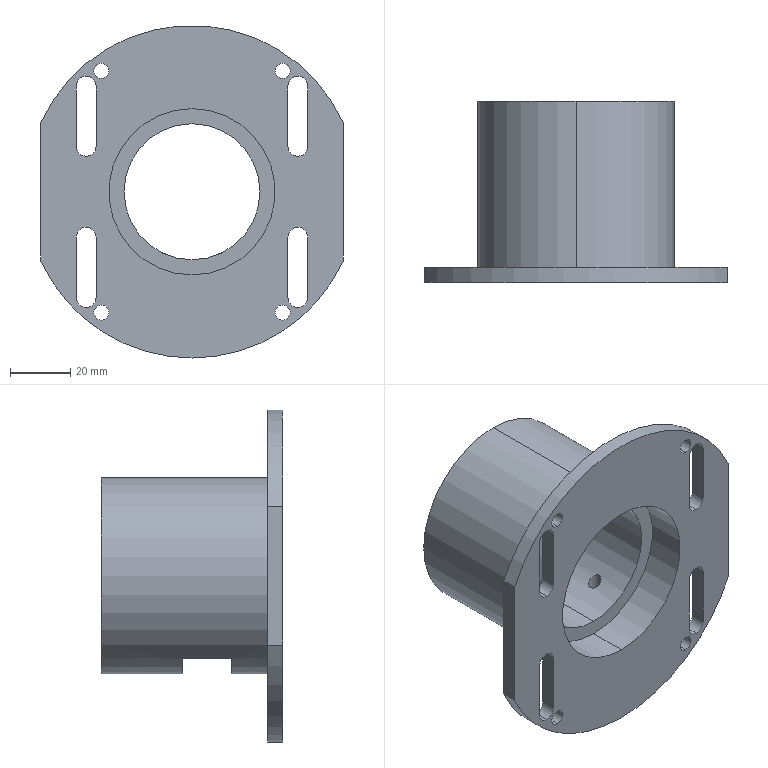Part | SolidWorks | features BaseBody 1 | 1 solid | 53 faces | box 100 x 60 x 110 mm | volume 106856 mm3 | cylinder 35 | plane 18 | commonest cylinder face diameters 6.5 x12 5 x8 4.2 x4 55 x4 110 x3 45 x2